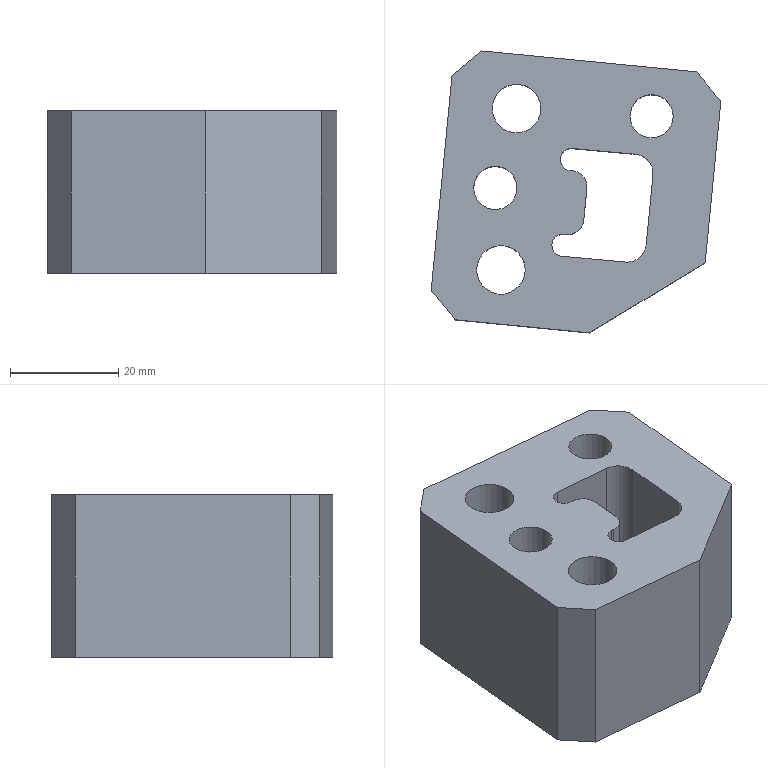Part | NX | features solid 2 | 1 solid | 30 faces | box 53.632 x 52.182 x 30 mm | volume 51476 mm3 | plane 18 | cylinder 6 | spline 6 | commonest cylinder face diameters 8 x2 9 x2 14 x2
STEP:
#1=CARTESIAN_POINT('',(-878.77,-144.615,108.));
#2=VERTEX_POINT('',#1);
#3=CARTESIAN_POINT('',(-876.165,-147.805,108.));
#4=VERTEX_POINT('',#3);
#5=CARTESIAN_POINT('',(-879.063,-147.547,108.));
#6=DIRECTION('',(0.,0.,1.));
#7=DIRECTION('',(-0.3864,-0.9223,0.));
#8=AXIS2_PLACEMENT_3D('',#5,#6,#7);
#9=ELLIPSE('',#8,2.95,2.906);
#10=EDGE_CURVE('',#2,#4,#9,.F.);
#11=ORIENTED_EDGE('',*,*,#10,.T.);
#12=CARTESIAN_POINT('',(-876.746,-153.745,108.));
#13=VERTEX_POINT('',#12);
#14=CARTESIAN_POINT('',(-873.886,-124.528,108.));
#15=DIRECTION('',(-0.09741,-0.9952,0.));
#16=VECTOR('',#15,1000.);
#17=LINE('',#14,#16);
#18=EDGE_CURVE('',#4,#13,#17,.T.);
#19=ORIENTED_EDGE('',*,*,#18,.T.);
#20=CARTESIAN_POINT('',(-879.938,-156.418,108.));
#21=VERTEX_POINT('',#20);
#22=CARTESIAN_POINT('',(-879.645,-153.487,108.));
#23=DIRECTION('',(0.,0.,1.));
#24=DIRECTION('',(-0.3864,-0.9223,0.));
#25=AXIS2_PLACEMENT_3D('',#22,#23,#24);
#26=ELLIPSE('',#25,2.95,2.906);
#27=EDGE_CURVE('',#13,#21,#26,.F.);
#28=ORIENTED_EDGE('',*,*,#27,.T.);
#29=CARTESIAN_POINT('',(-880.419,-156.374,108.));
#30=VERTEX_POINT('',#29);
#31=CARTESIAN_POINT('',(-838.877,-160.173,108.));
#32=DIRECTION('',(-0.9958,0.09106,0.));
#33=VECTOR('',#32,1000.);
#34=LINE('',#31,#33);
#35=EDGE_CURVE('',#21,#30,#34,.T.);
#36=ORIENTED_EDGE('',*,*,#35,.T.);
#37=CARTESIAN_POINT('',(-880.826,-160.449,108.));
#38=VERTEX_POINT('',#37);
#39=CARTESIAN_POINT('',(-880.622,-158.411,108.));
#40=DIRECTION('',(0.,0.,1.));
#41=DIRECTION('',(-0.3864,-0.9223,0.));
#42=AXIS2_PLACEMENT_3D('',#39,#40,#41);
#43=ELLIPSE('',#42,2.05,2.02);
#44=EDGE_CURVE('',#38,#30,#43,.F.);
#45=ORIENTED_EDGE('',*,*,#44,.F.);
#46=CARTESIAN_POINT('',(-869.041,-161.526,108.));
#47=VERTEX_POINT('',#46);
#48=CARTESIAN_POINT('',(-839.25,-164.25,108.));
#49=DIRECTION('',(-0.9958,0.09106,0.));
#50=VECTOR('',#49,1000.);
#51=LINE('',#48,#50);
#52=EDGE_CURVE('',#47,#38,#51,.T.);
#53=ORIENTED_EDGE('',*,*,#52,.F.);
#54=CARTESIAN_POINT('',(-865.2,-158.31,108.));
#55=VERTEX_POINT('',#54);
#56=CARTESIAN_POINT('',(-868.688,-157.998,108.));
#57=DIRECTION('',(0.,0.,1.));
#58=DIRECTION('',(-0.3864,-0.9223,0.));
#59=AXIS2_PLACEMENT_3D('',#56,#57,#58);
#60=ELLIPSE('',#59,3.55,3.497);
#61=EDGE_CURVE('',#55,#47,#60,.F.);
#62=ORIENTED_EDGE('',*,*,#61,.F.);
#63=CARTESIAN_POINT('',(-863.937,-145.412,108.));
#64=VERTEX_POINT('',#63);
#65=CARTESIAN_POINT('',(-862.007,-125.691,108.));
#66=DIRECTION('',(-0.09741,-0.9952,0.));
#67=VECTOR('',#66,1000.);
#68=LINE('',#65,#67);
#69=EDGE_CURVE('',#64,#55,#68,.T.);
#70=ORIENTED_EDGE('',*,*,#69,.F.);
#71=CARTESIAN_POINT('',(-867.073,-141.573,108.));
#72=VERTEX_POINT('',#71);
#73=CARTESIAN_POINT('',(-867.426,-145.101,108.));
#74=DIRECTION('',(0.,0.,1.));
#75=DIRECTION('',(-0.3864,-0.9223,0.));
#76=AXIS2_PLACEMENT_3D('',#73,#74,#75);
#77=ELLIPSE('',#76,3.55,3.497);
#78=EDGE_CURVE('',#72,#64,#77,.F.);
#79=ORIENTED_EDGE('',*,*,#78,.F.);
#80=CARTESIAN_POINT('',(-878.865,-140.495,108.));
#81=VERTEX_POINT('',#80);
#82=CARTESIAN_POINT('',(-837.425,-144.284,108.));
#83=DIRECTION('',(-0.9958,0.09106,0.));
#84=VECTOR('',#83,1000.);
#85=LINE('',#82,#84);
#86=EDGE_CURVE('',#72,#81,#85,.T.);
#87=ORIENTED_EDGE('',*,*,#86,.T.);
#88=CARTESIAN_POINT('',(-879.272,-144.569,108.));
#89=VERTEX_POINT('',#88);
#90=CARTESIAN_POINT('',(-879.068,-142.532,108.));
#91=DIRECTION('',(0.,0.,1.));
#92=DIRECTION('',(-0.3864,-0.9223,0.));
#93=AXIS2_PLACEMENT_3D('',#90,#91,#92);
#94=ELLIPSE('',#93,2.05,2.02);
#95=EDGE_CURVE('',#89,#81,#94,.F.);
#96=ORIENTED_EDGE('',*,*,#95,.F.);
#97=CARTESIAN_POINT('',(-837.798,-148.361,108.));
#98=DIRECTION('',(-0.9958,0.09106,0.));
#99=VECTOR('',#98,1000.);
#100=LINE('',#97,#99);
#101=EDGE_CURVE('',#2,#89,#100,.T.);
#102=ORIENTED_EDGE('',*,*,#101,.F.);
#103=EDGE_LOOP('',(#11,#19,#28,#36,#45,#53,#62,#70,#79,#87,#96,#102));
#104=FACE_BOUND('',#103,.T.);
#105=CARTESIAN_POINT('',(-860.199,-134.54,108.));
#106=VERTEX_POINT('',#105);
#107=CARTESIAN_POINT('',(-864.199,-134.54,108.));
#108=DIRECTION('',(0.,0.,1.));
#109=DIRECTION('',(1.,0.,0.));
#110=AXIS2_PLACEMENT_3D('',#107,#108,#109);
#111=CIRCLE('',#110,4.);
#112=EDGE_CURVE('',#106,#106,#111,.T.);
#113=ORIENTED_EDGE('',*,*,#112,.T.);
#114=EDGE_LOOP('',(#113));
#115=FACE_BOUND('',#114,.T.);
#116=CARTESIAN_POINT('',(-895.677,-122.441,108.));
#117=VERTEX_POINT('',#116);
#118=CARTESIAN_POINT('',(-855.864,-126.307,108.));
#119=VERTEX_POINT('',#118);
#120=CARTESIAN_POINT('',(-905.63,-121.474,108.));
#121=DIRECTION('',(0.9953,-0.09666,0.));
#122=VECTOR('',#121,1000.);
#123=LINE('',#120,#122);
#124=EDGE_CURVE('',#117,#119,#123,.T.);
#125=ORIENTED_EDGE('',*,*,#124,.T.);
#126=CARTESIAN_POINT('',(-851.371,-131.767,108.));
#127=VERTEX_POINT('',#126);
#128=CARTESIAN_POINT('',(-855.864,-126.307,108.));
#129=DIRECTION('',(0.6354,-0.7721,0.));
#130=VECTOR('',#129,1000.);
#131=LINE('',#128,#130);
#132=EDGE_CURVE('',#119,#127,#131,.T.);
#133=ORIENTED_EDGE('',*,*,#132,.T.);
#134=CARTESIAN_POINT('',(-854.271,-161.627,108.));
#135=VERTEX_POINT('',#134);
#136=CARTESIAN_POINT('',(-850.888,-126.79,108.));
#137=DIRECTION('',(0.09666,0.9953,0.));
#138=VECTOR('',#137,1000.);
#139=LINE('',#136,#138);
#140=EDGE_CURVE('',#135,#127,#139,.T.);
#141=ORIENTED_EDGE('',*,*,#140,.F.);
#142=CARTESIAN_POINT('',(-875.627,-174.623,108.));
#143=VERTEX_POINT('',#142);
#144=CARTESIAN_POINT('',(-875.627,-174.623,108.));
#145=DIRECTION('',(0.8542,0.5199,0.));
#146=VECTOR('',#145,1000.);
#147=LINE('',#144,#146);
#148=EDGE_CURVE('',#143,#135,#147,.T.);
#149=ORIENTED_EDGE('',*,*,#148,.F.);
#150=CARTESIAN_POINT('',(-900.51,-172.207,108.));
#151=VERTEX_POINT('',#150);
#152=CARTESIAN_POINT('',(-910.463,-171.24,108.));
#153=DIRECTION('',(0.9953,-0.09666,0.));
#154=VECTOR('',#153,1000.);
#155=LINE('',#152,#154);
#156=EDGE_CURVE('',#151,#143,#155,.T.);
#157=ORIENTED_EDGE('',*,*,#156,.F.);
#158=CARTESIAN_POINT('',(-905.003,-166.747,108.));
#159=VERTEX_POINT('',#158);
#160=CARTESIAN_POINT('',(-905.003,-166.747,108.));
#161=DIRECTION('',(-0.6354,0.7721,0.));
#162=VECTOR('',#161,1000.);
#163=LINE('',#160,#162);
#164=EDGE_CURVE('',#151,#159,#163,.T.);
#165=ORIENTED_EDGE('',*,*,#164,.T.);
#166=CARTESIAN_POINT('',(-901.137,-126.934,108.));
#167=VERTEX_POINT('',#166);
#168=CARTESIAN_POINT('',(-900.653,-121.957,108.));
#169=DIRECTION('',(0.09666,0.9953,0.));
#170=VECTOR('',#169,1000.);
#171=LINE('',#168,#170);
#172=EDGE_CURVE('',#159,#167,#171,.T.);
#173=ORIENTED_EDGE('',*,*,#172,.T.);
#174=CARTESIAN_POINT('',(-895.677,-122.441,108.));
#175=DIRECTION('',(-0.7721,-0.6354,0.));
#176=VECTOR('',#175,1000.);
#177=LINE('',#174,#176);
#178=EDGE_CURVE('',#167,#117,#177,.F.);
#179=ORIENTED_EDGE('',*,*,#178,.T.);
#180=EDGE_LOOP('',(#125,#133,#141,#149,#157,#165,#173,#179));
#181=FACE_BOUND('',#180,.T.);
#182=CARTESIAN_POINT('',(-899.078,-162.978,108.));
#183=VERTEX_POINT('',#182);
#184=CARTESIAN_POINT('',(-892.078,-162.978,108.));
#185=DIRECTION('',(0.,0.,1.));
#186=DIRECTION('',(-1.,0.,0.));
#187=AXIS2_PLACEMENT_3D('',#184,#185,#186);
#188=CIRCLE('',#187,7.);
#189=EDGE_CURVE('',#183,#183,#188,.T.);
#190=ORIENTED_EDGE('',*,*,#189,.T.);
#191=EDGE_LOOP('',(#190));
#192=FACE_BOUND('',#191,.T.);
#193=CARTESIAN_POINT('',(-896.179,-133.119,108.));
#194=VERTEX_POINT('',#193);
#195=CARTESIAN_POINT('',(-889.179,-133.119,108.));
#196=DIRECTION('',(0.,0.,1.));
#197=DIRECTION('',(-1.,0.,0.));
#198=AXIS2_PLACEMENT_3D('',#195,#196,#197);
#199=CIRCLE('',#198,7.);
#200=EDGE_CURVE('',#194,#194,#199,.T.);
#201=ORIENTED_EDGE('',*,*,#200,.T.);
#202=EDGE_LOOP('',(#201));
#203=FACE_BOUND('',#202,.T.);
#204=CARTESIAN_POINT('',(-897.117,-147.807,108.));
#205=VERTEX_POINT('',#204);
#206=CARTESIAN_POINT('',(-893.117,-147.807,108.));
#207=DIRECTION('',(0.,0.,1.));
#208=DIRECTION('',(-1.,0.,0.));
#209=AXIS2_PLACEMENT_3D('',#206,#207,#208);
#210=CIRCLE('',#209,4.);
#211=EDGE_CURVE('',#205,#205,#210,.T.);
#212=ORIENTED_EDGE('',*,*,#211,.T.);
#213=EDGE_LOOP('',(#212));
#214=FACE_BOUND('',#213,.T.);
#215=CARTESIAN_POINT('',(-835.958,-128.24,108.));
#216=DIRECTION('',(0.,0.,1.));
#217=DIRECTION('',(-1.,0.,0.));
#218=AXIS2_PLACEMENT_3D('',#215,#216,#217);
#219=PLANE('',#218);
#220=ADVANCED_FACE('',(#104,#115,#181,#192,#203,#214),#219,.F.);
#221=CARTESIAN_POINT('',(-876.746,-153.745,138.));
#222=VERTEX_POINT('',#221);
#223=CARTESIAN_POINT('',(-876.165,-147.805,138.));
#224=VERTEX_POINT('',#223);
#225=CARTESIAN_POINT('',(-876.746,-153.745,138.));
#226=DIRECTION('',(0.09741,0.9952,0.));
#227=VECTOR('',#226,1000.);
#228=LINE('',#225,#227);
#229=EDGE_CURVE('',#222,#224,#228,.T.);
#230=ORIENTED_EDGE('',*,*,#229,.T.);
#231=CARTESIAN_POINT('',(-878.77,-144.615,138.));
#232=VERTEX_POINT('',#231);
#233=CARTESIAN_POINT('',(-879.063,-147.547,138.));
#234=DIRECTION('',(0.,0.,1.));
#235=DIRECTION('',(-0.3864,-0.9223,0.));
#236=AXIS2_PLACEMENT_3D('',#233,#234,#235);
#237=ELLIPSE('',#236,2.95,2.906);
#238=EDGE_CURVE('',#224,#232,#237,.T.);
#239=ORIENTED_EDGE('',*,*,#238,.T.);
#240=CARTESIAN_POINT('',(-879.272,-144.569,138.));
#241=VERTEX_POINT('',#240);
#242=CARTESIAN_POINT('',(-879.272,-144.569,138.));
#243=DIRECTION('',(0.9958,-0.09106,0.));
#244=VECTOR('',#243,1000.);
#245=LINE('',#242,#244);
#246=EDGE_CURVE('',#241,#232,#245,.T.);
#247=ORIENTED_EDGE('',*,*,#246,.F.);
#248=CARTESIAN_POINT('',(-878.865,-140.495,138.));
#249=VERTEX_POINT('',#248);
#250=CARTESIAN_POINT('',(-879.068,-142.532,138.));
#251=DIRECTION('',(0.,0.,1.));
#252=DIRECTION('',(-0.3864,-0.9223,0.));
#253=AXIS2_PLACEMENT_3D('',#250,#251,#252);
#254=ELLIPSE('',#253,2.05,2.02);
#255=EDGE_CURVE('',#249,#241,#254,.T.);
#256=ORIENTED_EDGE('',*,*,#255,.F.);
#257=CARTESIAN_POINT('',(-867.073,-141.573,138.));
#258=VERTEX_POINT('',#257);
#259=CARTESIAN_POINT('',(-878.865,-140.495,138.));
#260=DIRECTION('',(0.9958,-0.09106,0.));
#261=VECTOR('',#260,1000.);
#262=LINE('',#259,#261);
#263=EDGE_CURVE('',#249,#258,#262,.T.);
#264=ORIENTED_EDGE('',*,*,#263,.T.);
#265=CARTESIAN_POINT('',(-863.937,-145.412,138.));
#266=VERTEX_POINT('',#265);
#267=CARTESIAN_POINT('',(-867.426,-145.101,138.));
#268=DIRECTION('',(0.,0.,1.));
#269=DIRECTION('',(-0.3864,-0.9223,0.));
#270=AXIS2_PLACEMENT_3D('',#267,#268,#269);
#271=ELLIPSE('',#270,3.55,3.497);
#272=EDGE_CURVE('',#266,#258,#271,.T.);
#273=ORIENTED_EDGE('',*,*,#272,.F.);
#274=CARTESIAN_POINT('',(-865.2,-158.31,138.));
#275=VERTEX_POINT('',#274);
#276=CARTESIAN_POINT('',(-865.2,-158.31,138.));
#277=DIRECTION('',(0.09741,0.9952,0.));
#278=VECTOR('',#277,1000.);
#279=LINE('',#276,#278);
#280=EDGE_CURVE('',#275,#266,#279,.T.);
#281=ORIENTED_EDGE('',*,*,#280,.F.);
#282=CARTESIAN_POINT('',(-869.041,-161.526,138.));
#283=VERTEX_POINT('',#282);
#284=CARTESIAN_POINT('',(-868.688,-157.998,138.));
#285=DIRECTION('',(0.,0.,1.));
#286=DIRECTION('',(-0.3864,-0.9223,0.));
#287=AXIS2_PLACEMENT_3D('',#284,#285,#286);
#288=ELLIPSE('',#287,3.55,3.497);
#289=EDGE_CURVE('',#283,#275,#288,.T.);
#290=ORIENTED_EDGE('',*,*,#289,.F.);
#291=CARTESIAN_POINT('',(-880.826,-160.449,138.));
#292=VERTEX_POINT('',#291);
#293=CARTESIAN_POINT('',(-880.826,-160.449,138.));
#294=DIRECTION('',(0.9958,-0.09106,0.));
#295=VECTOR('',#294,1000.);
#296=LINE('',#293,#295);
#297=EDGE_CURVE('',#292,#283,#296,.T.);
#298=ORIENTED_EDGE('',*,*,#297,.F.);
#299=CARTESIAN_POINT('',(-880.419,-156.374,138.));
#300=VERTEX_POINT('',#299);
#301=CARTESIAN_POINT('',(-880.622,-158.411,138.));
#302=DIRECTION('',(0.,0.,1.));
#303=DIRECTION('',(-0.3864,-0.9223,0.));
#304=AXIS2_PLACEMENT_3D('',#301,#302,#303);
#305=ELLIPSE('',#304,2.05,2.02);
#306=EDGE_CURVE('',#300,#292,#305,.T.);
#307=ORIENTED_EDGE('',*,*,#306,.F.);
#308=CARTESIAN_POINT('',(-879.938,-156.418,138.));
#309=VERTEX_POINT('',#308);
#310=CARTESIAN_POINT('',(-880.419,-156.374,138.));
#311=DIRECTION('',(0.9958,-0.09106,0.));
#312=VECTOR('',#311,1000.);
#313=LINE('',#310,#312);
#314=EDGE_CURVE('',#300,#309,#313,.T.);
#315=ORIENTED_EDGE('',*,*,#314,.T.);
#316=CARTESIAN_POINT('',(-879.645,-153.487,138.));
#317=DIRECTION('',(0.,0.,1.));
#318=DIRECTION('',(-0.3864,-0.9223,0.));
#319=AXIS2_PLACEMENT_3D('',#316,#317,#318);
#320=ELLIPSE('',#319,2.95,2.906);
#321=EDGE_CURVE('',#309,#222,#320,.T.);
#322=ORIENTED_EDGE('',*,*,#321,.T.);
#323=EDGE_LOOP('',(#230,#239,#247,#256,#264,#273,#281,#290,#298,#307,#315,#322));
#324=FACE_BOUND('',#323,.T.);
#325=CARTESIAN_POINT('',(-854.271,-161.627,138.));
#326=VERTEX_POINT('',#325);
#327=CARTESIAN_POINT('',(-851.371,-131.767,138.));
#328=VERTEX_POINT('',#327);
#329=CARTESIAN_POINT('',(-850.888,-126.79,138.));
#330=DIRECTION('',(0.09666,0.9953,0.));
#331=VECTOR('',#330,1000.);
#332=LINE('',#329,#331);
#333=EDGE_CURVE('',#326,#328,#332,.T.);
#334=ORIENTED_EDGE('',*,*,#333,.T.);
#335=CARTESIAN_POINT('',(-855.864,-126.307,138.));
#336=VERTEX_POINT('',#335);
#337=CARTESIAN_POINT('',(-846.878,-137.227,138.));
#338=DIRECTION('',(-0.6354,0.7721,0.));
#339=VECTOR('',#338,1000.);
#340=LINE('',#337,#339);
#341=EDGE_CURVE('',#328,#336,#340,.T.);
#342=ORIENTED_EDGE('',*,*,#341,.T.);
#343=CARTESIAN_POINT('',(-895.677,-122.441,138.));
#344=VERTEX_POINT('',#343);
#345=CARTESIAN_POINT('',(-905.63,-121.474,138.));
#346=DIRECTION('',(0.9953,-0.09666,0.));
#347=VECTOR('',#346,1000.);
#348=LINE('',#345,#347);
#349=EDGE_CURVE('',#344,#336,#348,.T.);
#350=ORIENTED_EDGE('',*,*,#349,.F.);
#351=CARTESIAN_POINT('',(-901.137,-126.934,138.));
#352=VERTEX_POINT('',#351);
#353=CARTESIAN_POINT('',(-862.917,-95.481,138.));
#354=DIRECTION('',(0.7721,0.6354,0.));
#355=VECTOR('',#354,1000.);
#356=LINE('',#353,#355);
#357=EDGE_CURVE('',#344,#352,#356,.F.);
#358=ORIENTED_EDGE('',*,*,#357,.T.);
#359=CARTESIAN_POINT('',(-905.003,-166.747,138.));
#360=VERTEX_POINT('',#359);
#361=CARTESIAN_POINT('',(-900.653,-121.957,138.));
#362=DIRECTION('',(0.09666,0.9953,0.));
#363=VECTOR('',#362,1000.);
#364=LINE('',#361,#363);
#365=EDGE_CURVE('',#360,#352,#364,.T.);
#366=ORIENTED_EDGE('',*,*,#365,.F.);
#367=CARTESIAN_POINT('',(-900.51,-172.207,138.));
#368=VERTEX_POINT('',#367);
#369=CARTESIAN_POINT('',(-896.016,-177.667,138.));
#370=DIRECTION('',(0.6354,-0.7721,0.));
#371=VECTOR('',#370,1000.);
#372=LINE('',#369,#371);
#373=EDGE_CURVE('',#360,#368,#372,.T.);
#374=ORIENTED_EDGE('',*,*,#373,.T.);
#375=CARTESIAN_POINT('',(-875.627,-174.623,138.));
#376=VERTEX_POINT('',#375);
#377=CARTESIAN_POINT('',(-910.463,-171.24,138.));
#378=DIRECTION('',(0.9953,-0.09666,0.));
#379=VECTOR('',#378,1000.);
#380=LINE('',#377,#379);
#381=EDGE_CURVE('',#368,#376,#380,.T.);
#382=ORIENTED_EDGE('',*,*,#381,.T.);
#383=CARTESIAN_POINT('',(-826.08,-144.471,138.));
#384=DIRECTION('',(-0.8542,-0.5199,0.));
#385=VECTOR('',#384,1000.);
#386=LINE('',#383,#385);
#387=EDGE_CURVE('',#326,#376,#386,.T.);
#388=ORIENTED_EDGE('',*,*,#387,.F.);
#389=EDGE_LOOP('',(#334,#342,#350,#358,#366,#374,#382,#388));
#390=FACE_BOUND('',#389,.T.);
#391=CARTESIAN_POINT('',(-860.199,-134.54,138.));
#392=VERTEX_POINT('',#391);
#393=CARTESIAN_POINT('',(-864.199,-134.54,138.));
#394=DIRECTION('',(0.,0.,1.));
#395=DIRECTION('',(1.,0.,0.));
#396=AXIS2_PLACEMENT_3D('',#393,#394,#395);
#397=CIRCLE('',#396,4.);
#398=EDGE_CURVE('',#392,#392,#397,.F.);
#399=ORIENTED_EDGE('',*,*,#398,.T.);
#400=EDGE_LOOP('',(#399));
#401=FACE_BOUND('',#400,.T.);
#402=CARTESIAN_POINT('',(-896.578,-162.978,138.));
#403=VERTEX_POINT('',#402);
#404=CARTESIAN_POINT('',(-892.078,-162.978,138.));
#405=DIRECTION('',(0.,0.,1.));
#406=DIRECTION('',(-1.,0.,0.));
#407=AXIS2_PLACEMENT_3D('',#404,#405,#406);
#408=CIRCLE('',#407,4.5);
#409=EDGE_CURVE('',#403,#403,#408,.T.);
#410=ORIENTED_EDGE('',*,*,#409,.F.);
#411=EDGE_LOOP('',(#410));
#412=FACE_BOUND('',#411,.T.);
#413=CARTESIAN_POINT('',(-893.679,-133.119,138.));
#414=VERTEX_POINT('',#413);
#415=CARTESIAN_POINT('',(-889.179,-133.119,138.));
#416=DIRECTION('',(0.,0.,1.));
#417=DIRECTION('',(-1.,0.,0.));
#418=AXIS2_PLACEMENT_3D('',#415,#416,#417);
#419=CIRCLE('',#418,4.5);
#420=EDGE_CURVE('',#414,#414,#419,.T.);
#421=ORIENTED_EDGE('',*,*,#420,.F.);
#422=EDGE_LOOP('',(#421));
#423=FACE_BOUND('',#422,.T.);
#424=CARTESIAN_POINT('',(-897.117,-147.807,138.));
#425=VERTEX_POINT('',#424);
#426=CARTESIAN_POINT('',(-893.117,-147.807,138.));
#427=DIRECTION('',(0.,0.,1.));
#428=DIRECTION('',(-1.,0.,0.));
#429=AXIS2_PLACEMENT_3D('',#426,#427,#428);
#430=CIRCLE('',#429,4.);
#431=EDGE_CURVE('',#425,#425,#430,.T.);
#432=ORIENTED_EDGE('',*,*,#431,.F.);
#433=EDGE_LOOP('',(#432));
#434=FACE_BOUND('',#433,.T.);
#435=CARTESIAN_POINT('',(-835.958,-128.24,138.));
#436=DIRECTION('',(0.,0.,1.));
#437=DIRECTION('',(-1.,0.,0.));
#438=AXIS2_PLACEMENT_3D('',#435,#436,#437);
#439=PLANE('',#438);
#440=ADVANCED_FACE('',(#324,#390,#401,#412,#423,#434),#439,.T.);
#441=ORIENTED_EDGE('',*,*,#349,.T.);
#442=CARTESIAN_POINT('',(-855.864,-126.307,108.));
#443=DIRECTION('',(0.,0.,-1.));
#444=VECTOR('',#443,1000.);
#445=LINE('',#442,#444);
#446=EDGE_CURVE('',#336,#119,#445,.T.);
#447=ORIENTED_EDGE('',*,*,#446,.T.);
#448=ORIENTED_EDGE('',*,*,#124,.F.);
#449=CARTESIAN_POINT('',(-895.677,-122.441,108.));
#450=DIRECTION('',(0.,0.,1.));
#451=VECTOR('',#450,1000.);
#452=LINE('',#449,#451);
#453=EDGE_CURVE('',#117,#344,#452,.T.);
#454=ORIENTED_EDGE('',*,*,#453,.T.);
#455=EDGE_LOOP('',(#441,#447,#448,#454));
#456=FACE_BOUND('',#455,.T.);
#457=CARTESIAN_POINT('',(-900.653,-121.957,108.));
#458=DIRECTION('',(-0.09666,-0.9953,0.));
#459=DIRECTION('',(0.9953,-0.09666,0.));
#460=AXIS2_PLACEMENT_3D('',#457,#458,#459);
#461=PLANE('',#460);
#462=ADVANCED_FACE('',(#456),#461,.F.);
#463=ORIENTED_EDGE('',*,*,#140,.T.);
#464=CARTESIAN_POINT('',(-851.371,-131.767,138.));
#465=DIRECTION('',(0.,0.,1.));
#466=VECTOR('',#465,1000.);
#467=LINE('',#464,#466);
#468=EDGE_CURVE('',#127,#328,#467,.T.);
#469=ORIENTED_EDGE('',*,*,#468,.T.);
#470=ORIENTED_EDGE('',*,*,#333,.F.);
#471=CARTESIAN_POINT('',(-854.271,-161.627,308.));
#472=DIRECTION('',(0.,0.,-1.));
#473=VECTOR('',#472,1000.);
#474=LINE('',#471,#473);
#475=EDGE_CURVE('',#326,#135,#474,.T.);
#476=ORIENTED_EDGE('',*,*,#475,.T.);
#477=EDGE_LOOP('',(#463,#469,#470,#476));
#478=FACE_BOUND('',#477,.T.);
#479=CARTESIAN_POINT('',(-855.72,-176.556,108.));
#480=DIRECTION('',(0.9953,-0.09666,0.));
#481=DIRECTION('',(0.09666,0.9953,0.));
#482=AXIS2_PLACEMENT_3D('',#479,#480,#481);
#483=PLANE('',#482);
#484=ADVANCED_FACE('',(#478),#483,.T.);
#485=CARTESIAN_POINT('',(-875.627,-174.623,308.));
#486=DIRECTION('',(0.,0.,-1.));
#487=VECTOR('',#486,1000.);
#488=LINE('',#485,#487);
#489=EDGE_CURVE('',#376,#143,#488,.T.);
#490=ORIENTED_EDGE('',*,*,#489,.F.);
#491=ORIENTED_EDGE('',*,*,#381,.F.);
#492=CARTESIAN_POINT('',(-900.51,-172.207,108.));
#493=DIRECTION('',(0.,0.,-1.));
#494=VECTOR('',#493,1000.);
#495=LINE('',#492,#494);
#496=EDGE_CURVE('',#368,#151,#495,.T.);
#497=ORIENTED_EDGE('',*,*,#496,.T.);
#498=ORIENTED_EDGE('',*,*,#156,.T.);
#499=EDGE_LOOP('',(#490,#491,#497,#498));
#500=FACE_BOUND('',#499,.T.);
#501=CARTESIAN_POINT('',(-905.486,-171.723,108.));
#502=DIRECTION('',(-0.09666,-0.9953,0.));
#503=DIRECTION('',(0.9953,-0.09666,0.));
#504=AXIS2_PLACEMENT_3D('',#501,#502,#503);
#505=PLANE('',#504);
#506=ADVANCED_FACE('',(#500),#505,.T.);
#507=ORIENTED_EDGE('',*,*,#172,.F.);
#508=CARTESIAN_POINT('',(-905.003,-166.747,138.));
#509=DIRECTION('',(0.,0.,1.));
#510=VECTOR('',#509,1000.);
#511=LINE('',#508,#510);
#512=EDGE_CURVE('',#159,#360,#511,.T.);
#513=ORIENTED_EDGE('',*,*,#512,.T.);
#514=ORIENTED_EDGE('',*,*,#365,.T.);
#515=CARTESIAN_POINT('',(-901.137,-126.934,108.));
#516=DIRECTION('',(0.,0.,-1.));
#517=VECTOR('',#516,1000.);
#518=LINE('',#515,#517);
#519=EDGE_CURVE('',#352,#167,#518,.T.);
#520=ORIENTED_EDGE('',*,*,#519,.T.);
#521=EDGE_LOOP('',(#507,#513,#514,#520));
#522=FACE_BOUND('',#521,.T.);
#523=CARTESIAN_POINT('',(-905.486,-171.723,108.));
#524=DIRECTION('',(0.9953,-0.09666,0.));
#525=DIRECTION('',(0.09666,0.9953,0.));
#526=AXIS2_PLACEMENT_3D('',#523,#524,#525);
#527=PLANE('',#526);
#528=ADVANCED_FACE('',(#522),#527,.F.);
#529=CARTESIAN_POINT('',(-885.209,-164.325,123.));
#530=VERTEX_POINT('',#529);
#531=CARTESIAN_POINT('',(-892.078,-162.978,123.));
#532=DIRECTION('',(0.,0.,-1.));
#533=DIRECTION('',(0.9813,-0.1924,0.));
#534=AXIS2_PLACEMENT_3D('',#531,#532,#533);
#535=CIRCLE('',#534,7.);
#536=EDGE_CURVE('',#530,#530,#535,.T.);
#537=ORIENTED_EDGE('',*,*,#536,.F.);
#538=EDGE_LOOP('',(#537));
#539=FACE_BOUND('',#538,.T.);
#540=ORIENTED_EDGE('',*,*,#189,.F.);
#541=EDGE_LOOP('',(#540));
#542=FACE_BOUND('',#541,.T.);
#543=CARTESIAN_POINT('',(-892.078,-162.978,123.));
#544=DIRECTION('',(0.,0.,-1.));
#545=DIRECTION('',(0.9813,-0.1924,0.));
#546=AXIS2_PLACEMENT_3D('',#543,#544,#545);
#547=CYLINDRICAL_SURFACE('',#546,7.);
#548=ADVANCED_FACE('',(#539,#542),#547,.F.);
#549=CARTESIAN_POINT('',(-896.578,-162.978,123.));
#550=VERTEX_POINT('',#549);
#551=CARTESIAN_POINT('',(-892.078,-162.978,123.));
#552=DIRECTION('',(0.,0.,1.));
#553=DIRECTION('',(-1.,0.,0.));
#554=AXIS2_PLACEMENT_3D('',#551,#552,#553);
#555=CIRCLE('',#554,4.5);
#556=EDGE_CURVE('',#550,#550,#555,.T.);
#557=ORIENTED_EDGE('',*,*,#556,.T.);
#558=EDGE_LOOP('',(#557));
#559=FACE_BOUND('',#558,.T.);
#560=ORIENTED_EDGE('',*,*,#536,.T.);
#561=EDGE_LOOP('',(#560));
#562=FACE_BOUND('',#561,.T.);
#563=CARTESIAN_POINT('',(-892.078,-162.978,123.));
#564=DIRECTION('',(0.,0.,1.));
#565=DIRECTION('',(-0.9813,0.1924,0.));
#566=AXIS2_PLACEMENT_3D('',#563,#564,#565);
#567=PLANE('',#566);
#568=ADVANCED_FACE('',(#559,#562),#567,.F.);
#569=ORIENTED_EDGE('',*,*,#409,.T.);
#570=EDGE_LOOP('',(#569));
#571=FACE_BOUND('',#570,.T.);
#572=ORIENTED_EDGE('',*,*,#556,.F.);
#573=EDGE_LOOP('',(#572));
#574=FACE_BOUND('',#573,.T.);
#575=CARTESIAN_POINT('',(-892.078,-162.978,123.));
#576=DIRECTION('',(0.,0.,1.));
#577=DIRECTION('',(-0.9813,0.1924,0.));
#578=AXIS2_PLACEMENT_3D('',#575,#576,#577);
#579=CYLINDRICAL_SURFACE('',#578,4.5);
#580=ADVANCED_FACE('',(#571,#574),#579,.F.);
#581=CARTESIAN_POINT('',(-882.309,-134.466,123.));
#582=VERTEX_POINT('',#581);
#583=CARTESIAN_POINT('',(-889.179,-133.119,123.));
#584=DIRECTION('',(0.,0.,-1.));
#585=DIRECTION('',(0.9813,-0.1924,0.));
#586=AXIS2_PLACEMENT_3D('',#583,#584,#585);
#587=CIRCLE('',#586,7.);
#588=EDGE_CURVE('',#582,#582,#587,.T.);
#589=ORIENTED_EDGE('',*,*,#588,.F.);
#590=EDGE_LOOP('',(#589));
#591=FACE_BOUND('',#590,.T.);
#592=ORIENTED_EDGE('',*,*,#200,.F.);
#593=EDGE_LOOP('',(#592));
#594=FACE_BOUND('',#593,.T.);
#595=CARTESIAN_POINT('',(-889.179,-133.119,123.));
#596=DIRECTION('',(0.,0.,-1.));
#597=DIRECTION('',(0.9813,-0.1924,0.));
#598=AXIS2_PLACEMENT_3D('',#595,#596,#597);
#599=CYLINDRICAL_SURFACE('',#598,7.);
#600=ADVANCED_FACE('',(#591,#594),#599,.F.);
#601=CARTESIAN_POINT('',(-893.679,-133.119,123.));
#602=VERTEX_POINT('',#601);
#603=CARTESIAN_POINT('',(-889.179,-133.119,123.));
#604=DIRECTION('',(0.,0.,1.));
#605=DIRECTION('',(-1.,0.,0.));
#606=AXIS2_PLACEMENT_3D('',#603,#604,#605);
#607=CIRCLE('',#606,4.5);
#608=EDGE_CURVE('',#602,#602,#607,.T.);
#609=ORIENTED_EDGE('',*,*,#608,.T.);
#610=EDGE_LOOP('',(#609));
#611=FACE_BOUND('',#610,.T.);
#612=ORIENTED_EDGE('',*,*,#588,.T.);
#613=EDGE_LOOP('',(#612));
#614=FACE_BOUND('',#613,.T.);
#615=CARTESIAN_POINT('',(-889.179,-133.119,123.));
#616=DIRECTION('',(0.,0.,1.));
#617=DIRECTION('',(-0.9813,0.1924,0.));
#618=AXIS2_PLACEMENT_3D('',#615,#616,#617);
#619=PLANE('',#618);
#620=ADVANCED_FACE('',(#611,#614),#619,.F.);
#621=ORIENTED_EDGE('',*,*,#420,.T.);
#622=EDGE_LOOP('',(#621));
#623=FACE_BOUND('',#622,.T.);
#624=ORIENTED_EDGE('',*,*,#608,.F.);
#625=EDGE_LOOP('',(#624));
#626=FACE_BOUND('',#625,.T.);
#627=CARTESIAN_POINT('',(-889.179,-133.119,123.));
#628=DIRECTION('',(0.,0.,1.));
#629=DIRECTION('',(-0.9813,0.1924,0.));
#630=AXIS2_PLACEMENT_3D('',#627,#628,#629);
#631=CYLINDRICAL_SURFACE('',#630,4.5);
#632=ADVANCED_FACE('',(#623,#626),#631,.F.);
#633=ORIENTED_EDGE('',*,*,#431,.T.);
#634=EDGE_LOOP('',(#633));
#635=FACE_BOUND('',#634,.T.);
#636=ORIENTED_EDGE('',*,*,#211,.F.);
#637=EDGE_LOOP('',(#636));
#638=FACE_BOUND('',#637,.T.);
#639=CARTESIAN_POINT('',(-893.117,-147.807,148.));
#640=DIRECTION('',(0.,0.,-1.));
#641=DIRECTION('',(1.,0.,0.));
#642=AXIS2_PLACEMENT_3D('',#639,#640,#641);
#643=CYLINDRICAL_SURFACE('',#642,4.);
#644=ADVANCED_FACE('',(#635,#638),#643,.F.);
#645=ORIENTED_EDGE('',*,*,#164,.F.);
#646=ORIENTED_EDGE('',*,*,#496,.F.);
#647=ORIENTED_EDGE('',*,*,#373,.F.);
#648=ORIENTED_EDGE('',*,*,#512,.F.);
#649=EDGE_LOOP('',(#645,#646,#647,#648));
#650=FACE_BOUND('',#649,.T.);
#651=CARTESIAN_POINT('',(-905.003,-166.747,108.));
#652=DIRECTION('',(-0.7721,-0.6354,0.));
#653=DIRECTION('',(0.6354,-0.7721,0.));
#654=AXIS2_PLACEMENT_3D('',#651,#652,#653);
#655=PLANE('',#654);
#656=ADVANCED_FACE('',(#650),#655,.T.);
#657=ORIENTED_EDGE('',*,*,#178,.F.);
#658=ORIENTED_EDGE('',*,*,#519,.F.);
#659=ORIENTED_EDGE('',*,*,#357,.F.);
#660=ORIENTED_EDGE('',*,*,#453,.F.);
#661=EDGE_LOOP('',(#657,#658,#659,#660));
#662=FACE_BOUND('',#661,.T.);
#663=CARTESIAN_POINT('',(-895.677,-122.441,108.));
#664=DIRECTION('',(0.6354,-0.7721,0.));
#665=DIRECTION('',(0.7721,0.6354,0.));
#666=AXIS2_PLACEMENT_3D('',#663,#664,#665);
#667=PLANE('',#666);
#668=ADVANCED_FACE('',(#662),#667,.F.);
#669=ORIENTED_EDGE('',*,*,#398,.F.);
#670=EDGE_LOOP('',(#669));
#671=FACE_BOUND('',#670,.T.);
#672=ORIENTED_EDGE('',*,*,#112,.F.);
#673=EDGE_LOOP('',(#672));
#674=FACE_BOUND('',#673,.T.);
#675=CARTESIAN_POINT('',(-864.199,-134.54,188.));
#676=DIRECTION('',(0.,0.,-1.));
#677=DIRECTION('',(1.,0.,0.));
#678=AXIS2_PLACEMENT_3D('',#675,#676,#677);
#679=CYLINDRICAL_SURFACE('',#678,4.);
#680=ADVANCED_FACE('',(#671,#674),#679,.F.);
#681=ORIENTED_EDGE('',*,*,#387,.T.);
#682=ORIENTED_EDGE('',*,*,#489,.T.);
#683=ORIENTED_EDGE('',*,*,#148,.T.);
#684=ORIENTED_EDGE('',*,*,#475,.F.);
#685=EDGE_LOOP('',(#681,#682,#683,#684));
#686=FACE_BOUND('',#685,.T.);
#687=CARTESIAN_POINT('',(-875.627,-174.623,308.));
#688=DIRECTION('',(-0.5199,0.8542,0.));
#689=DIRECTION('',(-0.8542,-0.5199,0.));
#690=AXIS2_PLACEMENT_3D('',#687,#688,#689);
#691=PLANE('',#690);
#692=ADVANCED_FACE('',(#686),#691,.F.);
#693=ORIENTED_EDGE('',*,*,#341,.F.);
#694=ORIENTED_EDGE('',*,*,#468,.F.);
#695=ORIENTED_EDGE('',*,*,#132,.F.);
#696=ORIENTED_EDGE('',*,*,#446,.F.);
#697=EDGE_LOOP('',(#693,#694,#695,#696));
#698=FACE_BOUND('',#697,.T.);
#699=CARTESIAN_POINT('',(-855.864,-126.307,108.));
#700=DIRECTION('',(0.7721,0.6354,0.));
#701=DIRECTION('',(-0.6354,0.7721,0.));
#702=AXIS2_PLACEMENT_3D('',#699,#700,#701);
#703=PLANE('',#702);
#704=ADVANCED_FACE('',(#698),#703,.T.);
#705=CARTESIAN_POINT('',(-876.165,-147.805,211.));
#706=DIRECTION('',(0.,0.,-1.));
#707=VECTOR('',#706,1000.);
#708=LINE('',#705,#707);
#709=EDGE_CURVE('',#224,#4,#708,.T.);
#710=ORIENTED_EDGE('',*,*,#709,.F.);
#711=ORIENTED_EDGE('',*,*,#229,.F.);
#712=CARTESIAN_POINT('',(-876.746,-153.745,211.));
#713=DIRECTION('',(0.,0.,-1.));
#714=VECTOR('',#713,1000.);
#715=LINE('',#712,#714);
#716=EDGE_CURVE('',#222,#13,#715,.T.);
#717=ORIENTED_EDGE('',*,*,#716,.T.);
#718=ORIENTED_EDGE('',*,*,#18,.F.);
#719=EDGE_LOOP('',(#710,#711,#717,#718));
#720=FACE_BOUND('',#719,.T.);
#721=CARTESIAN_POINT('',(-876.746,-153.745,211.));
#722=DIRECTION('',(-0.9952,0.09741,0.));
#723=DIRECTION('',(-0.09741,-0.9952,0.));
#724=AXIS2_PLACEMENT_3D('',#721,#722,#723);
#725=PLANE('',#724);
#726=ADVANCED_FACE('',(#720),#725,.F.);
#727=ORIENTED_EDGE('',*,*,#716,.F.);
#728=ORIENTED_EDGE('',*,*,#321,.F.);
#729=CARTESIAN_POINT('',(-879.938,-156.418,211.));
#730=DIRECTION('',(0.,0.,-1.));
#731=VECTOR('',#730,1000.);
#732=LINE('',#729,#731);
#733=EDGE_CURVE('',#309,#21,#732,.T.);
#734=ORIENTED_EDGE('',*,*,#733,.T.);
#735=ORIENTED_EDGE('',*,*,#27,.F.);
#736=EDGE_LOOP('',(#727,#728,#734,#735));
#737=FACE_BOUND('',#736,.T.);
#738=CARTESIAN_POINT('',(-879.938,-156.418,138.));
#739=CARTESIAN_POINT('',(-879.938,-156.418,108.));
#740=CARTESIAN_POINT('',(-879.174,-156.488,138.));
#741=CARTESIAN_POINT('',(-879.174,-156.488,108.));
#742=CARTESIAN_POINT('',(-877.587,-155.982,138.));
#743=CARTESIAN_POINT('',(-877.587,-155.982,108.));
#744=CARTESIAN_POINT('',(-876.812,-154.492,138.));
#745=CARTESIAN_POINT('',(-876.812,-154.492,108.));
#746=CARTESIAN_POINT('',(-876.744,-153.718,138.));
#747=CARTESIAN_POINT('',(-876.744,-153.718,108.));
#748=B_SPLINE_SURFACE_WITH_KNOTS('',3,1,((#738,#739),(#740,#741),(#742,#743),(#744,#745),(#746,#747)),.SURF_OF_LINEAR_EXTRUSION.,.F.,.F.,.F.,(4,1,4),(2,2),(0.3012,1.092,1.884),(0.,1.),.UNSPECIFIED.);
#749=ADVANCED_FACE('',(#737),#748,.F.);
#750=ORIENTED_EDGE('',*,*,#733,.F.);
#751=ORIENTED_EDGE('',*,*,#314,.F.);
#752=CARTESIAN_POINT('',(-880.419,-156.374,211.));
#753=DIRECTION('',(0.,0.,-1.));
#754=VECTOR('',#753,1000.);
#755=LINE('',#752,#754);
#756=EDGE_CURVE('',#300,#30,#755,.T.);
#757=ORIENTED_EDGE('',*,*,#756,.T.);
#758=ORIENTED_EDGE('',*,*,#35,.F.);
#759=EDGE_LOOP('',(#750,#751,#757,#758));
#760=FACE_BOUND('',#759,.T.);
#761=CARTESIAN_POINT('',(-880.419,-156.374,211.));
#762=DIRECTION('',(0.09106,0.9958,0.));
#763=DIRECTION('',(-0.9958,0.09106,0.));
#764=AXIS2_PLACEMENT_3D('',#761,#762,#763);
#765=PLANE('',#764);
#766=ADVANCED_FACE('',(#760),#765,.F.);
#767=ORIENTED_EDGE('',*,*,#44,.T.);
#768=ORIENTED_EDGE('',*,*,#756,.F.);
#769=ORIENTED_EDGE('',*,*,#306,.T.);
#770=CARTESIAN_POINT('',(-880.826,-160.449,211.));
#771=DIRECTION('',(0.,0.,-1.));
#772=VECTOR('',#771,1000.);
#773=LINE('',#770,#772);
#774=EDGE_CURVE('',#292,#38,#773,.T.);
#775=ORIENTED_EDGE('',*,*,#774,.T.);
#776=EDGE_LOOP('',(#767,#768,#769,#775));
#777=FACE_BOUND('',#776,.T.);
#778=CARTESIAN_POINT('',(-880.381,-156.378,138.));
#779=CARTESIAN_POINT('',(-880.381,-156.378,108.));
#780=CARTESIAN_POINT('',(-880.91,-156.319,138.));
#781=CARTESIAN_POINT('',(-880.91,-156.319,108.));
#782=CARTESIAN_POINT('',(-882.017,-156.648,138.));
#783=CARTESIAN_POINT('',(-882.017,-156.648,108.));
#784=CARTESIAN_POINT('',(-882.855,-158.186,138.));
#785=CARTESIAN_POINT('',(-882.855,-158.186,108.));
#786=CARTESIAN_POINT('',(-882.368,-159.857,138.));
#787=CARTESIAN_POINT('',(-882.368,-159.857,108.));
#788=CARTESIAN_POINT('',(-881.357,-160.4,138.));
#789=CARTESIAN_POINT('',(-881.357,-160.4,108.));
#790=CARTESIAN_POINT('',(-880.826,-160.449,138.));
#791=CARTESIAN_POINT('',(-880.826,-160.449,108.));
#792=B_SPLINE_SURFACE_WITH_KNOTS('',3,1,((#778,#779),(#780,#781),(#782,#783),(#784,#785),(#786,#787),(#788,#789),(#790,#791)),.SURF_OF_LINEAR_EXTRUSION.,.F.,.F.,.F.,(4,1,1,1,4),(2,2),(3.424,4.214,5.004,5.794,6.584),(0.,1.),.UNSPECIFIED.);
#793=ADVANCED_FACE('',(#777),#792,.T.);
#794=ORIENTED_EDGE('',*,*,#52,.T.);
#795=ORIENTED_EDGE('',*,*,#774,.F.);
#796=ORIENTED_EDGE('',*,*,#297,.T.);
#797=CARTESIAN_POINT('',(-869.041,-161.526,211.));
#798=DIRECTION('',(0.,0.,-1.));
#799=VECTOR('',#798,1000.);
#800=LINE('',#797,#799);
#801=EDGE_CURVE('',#283,#47,#800,.T.);
#802=ORIENTED_EDGE('',*,*,#801,.T.);
#803=EDGE_LOOP('',(#794,#795,#796,#802));
#804=FACE_BOUND('',#803,.T.);
#805=CARTESIAN_POINT('',(-880.826,-160.449,211.));
#806=DIRECTION('',(0.09106,0.9958,0.));
#807=DIRECTION('',(-0.9958,0.09106,0.));
#808=AXIS2_PLACEMENT_3D('',#805,#806,#807);
#809=PLANE('',#808);
#810=ADVANCED_FACE('',(#804),#809,.T.);
#811=ORIENTED_EDGE('',*,*,#61,.T.);
#812=ORIENTED_EDGE('',*,*,#801,.F.);
#813=ORIENTED_EDGE('',*,*,#289,.T.);
#814=CARTESIAN_POINT('',(-865.2,-158.31,211.));
#815=DIRECTION('',(0.,0.,-1.));
#816=VECTOR('',#815,1000.);
#817=LINE('',#814,#816);
#818=EDGE_CURVE('',#275,#55,#817,.T.);
#819=ORIENTED_EDGE('',*,*,#818,.T.);
#820=EDGE_LOOP('',(#811,#812,#813,#819));
#821=FACE_BOUND('',#820,.T.);
#822=CARTESIAN_POINT('',(-869.074,-161.523,138.));
#823=CARTESIAN_POINT('',(-869.074,-161.523,108.));
#824=CARTESIAN_POINT('',(-868.155,-161.616,138.));
#825=CARTESIAN_POINT('',(-868.155,-161.616,108.));
#826=CARTESIAN_POINT('',(-866.24,-161.025,138.));
#827=CARTESIAN_POINT('',(-866.24,-161.025,108.));
#828=CARTESIAN_POINT('',(-865.291,-159.24,138.));
#829=CARTESIAN_POINT('',(-865.291,-159.24,108.));
#830=CARTESIAN_POINT('',(-865.2,-158.31,138.));
#831=CARTESIAN_POINT('',(-865.2,-158.31,108.));
#832=B_SPLINE_SURFACE_WITH_KNOTS('',3,1,((#822,#823),(#824,#825),(#826,#827),(#828,#829),(#830,#831)),.SURF_OF_LINEAR_EXTRUSION.,.F.,.F.,.F.,(4,1,4),(2,2),(0.2918,1.083,1.874),(0.,1.),.UNSPECIFIED.);
#833=ADVANCED_FACE('',(#821),#832,.T.);
#834=ORIENTED_EDGE('',*,*,#69,.T.);
#835=ORIENTED_EDGE('',*,*,#818,.F.);
#836=ORIENTED_EDGE('',*,*,#280,.T.);
#837=CARTESIAN_POINT('',(-863.937,-145.412,211.));
#838=DIRECTION('',(0.,0.,-1.));
#839=VECTOR('',#838,1000.);
#840=LINE('',#837,#839);
#841=EDGE_CURVE('',#266,#64,#840,.T.);
#842=ORIENTED_EDGE('',*,*,#841,.T.);
#843=EDGE_LOOP('',(#834,#835,#836,#842));
#844=FACE_BOUND('',#843,.T.);
#845=CARTESIAN_POINT('',(-865.2,-158.31,211.));
#846=DIRECTION('',(-0.9952,0.09741,0.));
#847=DIRECTION('',(-0.09741,-0.9952,0.));
#848=AXIS2_PLACEMENT_3D('',#845,#846,#847);
#849=PLANE('',#848);
#850=ADVANCED_FACE('',(#844),#849,.T.);
#851=ORIENTED_EDGE('',*,*,#78,.T.);
#852=ORIENTED_EDGE('',*,*,#841,.F.);
#853=ORIENTED_EDGE('',*,*,#272,.T.);
#854=CARTESIAN_POINT('',(-867.073,-141.573,211.));
#855=DIRECTION('',(0.,0.,-1.));
#856=VECTOR('',#855,1000.);
#857=LINE('',#854,#856);
#858=EDGE_CURVE('',#258,#72,#857,.T.);
#859=ORIENTED_EDGE('',*,*,#858,.T.);
#860=EDGE_LOOP('',(#851,#852,#853,#859));
#861=FACE_BOUND('',#860,.T.);
#862=CARTESIAN_POINT('',(-863.941,-145.445,138.));
#863=CARTESIAN_POINT('',(-863.941,-145.445,108.));
#864=CARTESIAN_POINT('',(-863.841,-144.518,138.));
#865=CARTESIAN_POINT('',(-863.841,-144.518,108.));
#866=CARTESIAN_POINT('',(-864.406,-142.596,138.));
#867=CARTESIAN_POINT('',(-864.406,-142.596,108.));
#868=CARTESIAN_POINT('',(-866.156,-141.657,138.));
#869=CARTESIAN_POINT('',(-866.156,-141.657,108.));
#870=CARTESIAN_POINT('',(-867.073,-141.573,138.));
#871=CARTESIAN_POINT('',(-867.073,-141.573,108.));
#872=B_SPLINE_SURFACE_WITH_KNOTS('',3,1,((#862,#863),(#864,#865),(#866,#867),(#868,#869),(#870,#871)),.SURF_OF_LINEAR_EXTRUSION.,.F.,.F.,.F.,(4,1,4),(2,2),(1.865,2.654,3.443),(0.,1.),.UNSPECIFIED.);
#873=ADVANCED_FACE('',(#861),#872,.T.);
#874=ORIENTED_EDGE('',*,*,#858,.F.);
#875=ORIENTED_EDGE('',*,*,#263,.F.);
#876=CARTESIAN_POINT('',(-878.865,-140.495,211.));
#877=DIRECTION('',(0.,0.,-1.));
#878=VECTOR('',#877,1000.);
#879=LINE('',#876,#878);
#880=EDGE_CURVE('',#249,#81,#879,.T.);
#881=ORIENTED_EDGE('',*,*,#880,.T.);
#882=ORIENTED_EDGE('',*,*,#86,.F.);
#883=EDGE_LOOP('',(#874,#875,#881,#882));
#884=FACE_BOUND('',#883,.T.);
#885=CARTESIAN_POINT('',(-878.865,-140.495,211.));
#886=DIRECTION('',(0.09106,0.9958,0.));
#887=DIRECTION('',(-0.9958,0.09106,0.));
#888=AXIS2_PLACEMENT_3D('',#885,#886,#887);
#889=PLANE('',#888);
#890=ADVANCED_FACE('',(#884),#889,.F.);
#891=ORIENTED_EDGE('',*,*,#95,.T.);
#892=ORIENTED_EDGE('',*,*,#880,.F.);
#893=ORIENTED_EDGE('',*,*,#255,.T.);
#894=CARTESIAN_POINT('',(-879.272,-144.569,211.));
#895=DIRECTION('',(0.,0.,-1.));
#896=VECTOR('',#895,1000.);
#897=LINE('',#894,#896);
#898=EDGE_CURVE('',#241,#89,#897,.T.);
#899=ORIENTED_EDGE('',*,*,#898,.T.);
#900=EDGE_LOOP('',(#891,#892,#893,#899));
#901=FACE_BOUND('',#900,.T.);
#902=CARTESIAN_POINT('',(-878.827,-140.499,138.));
#903=CARTESIAN_POINT('',(-878.827,-140.499,108.));
#904=CARTESIAN_POINT('',(-879.356,-140.44,138.));
#905=CARTESIAN_POINT('',(-879.356,-140.44,108.));
#906=CARTESIAN_POINT('',(-880.463,-140.769,138.));
#907=CARTESIAN_POINT('',(-880.463,-140.769,108.));
#908=CARTESIAN_POINT('',(-881.301,-142.306,138.));
#909=CARTESIAN_POINT('',(-881.301,-142.306,108.));
#910=CARTESIAN_POINT('',(-880.814,-143.978,138.));
#911=CARTESIAN_POINT('',(-880.814,-143.978,108.));
#912=CARTESIAN_POINT('',(-879.802,-144.521,138.));
#913=CARTESIAN_POINT('',(-879.802,-144.521,108.));
#914=CARTESIAN_POINT('',(-879.272,-144.569,138.));
#915=CARTESIAN_POINT('',(-879.272,-144.569,108.));
#916=B_SPLINE_SURFACE_WITH_KNOTS('',3,1,((#902,#903),(#904,#905),(#906,#907),(#908,#909),(#910,#911),(#912,#913),(#914,#915)),.SURF_OF_LINEAR_EXTRUSION.,.F.,.F.,.F.,(4,1,1,1,4),(2,2),(3.424,4.214,5.004,5.794,6.584),(0.,1.),.UNSPECIFIED.);
#917=ADVANCED_FACE('',(#901),#916,.T.);
#918=ORIENTED_EDGE('',*,*,#101,.T.);
#919=ORIENTED_EDGE('',*,*,#898,.F.);
#920=ORIENTED_EDGE('',*,*,#246,.T.);
#921=CARTESIAN_POINT('',(-878.77,-144.615,211.));
#922=DIRECTION('',(0.,0.,-1.));
#923=VECTOR('',#922,1000.);
#924=LINE('',#921,#923);
#925=EDGE_CURVE('',#232,#2,#924,.T.);
#926=ORIENTED_EDGE('',*,*,#925,.T.);
#927=EDGE_LOOP('',(#918,#919,#920,#926));
#928=FACE_BOUND('',#927,.T.);
#929=CARTESIAN_POINT('',(-879.272,-144.569,211.));
#930=DIRECTION('',(0.09106,0.9958,0.));
#931=DIRECTION('',(-0.9958,0.09106,0.));
#932=AXIS2_PLACEMENT_3D('',#929,#930,#931);
#933=PLANE('',#932);
#934=ADVANCED_FACE('',(#928),#933,.T.);
#935=ORIENTED_EDGE('',*,*,#925,.F.);
#936=ORIENTED_EDGE('',*,*,#238,.F.);
#937=ORIENTED_EDGE('',*,*,#709,.T.);
#938=ORIENTED_EDGE('',*,*,#10,.F.);
#939=EDGE_LOOP('',(#935,#936,#937,#938));
#940=FACE_BOUND('',#939,.T.);
#941=CARTESIAN_POINT('',(-876.165,-147.805,138.));
#942=CARTESIAN_POINT('',(-876.165,-147.805,108.));
#943=CARTESIAN_POINT('',(-876.089,-147.034,138.));
#944=CARTESIAN_POINT('',(-876.089,-147.034,108.));
#945=CARTESIAN_POINT('',(-876.573,-145.441,138.));
#946=CARTESIAN_POINT('',(-876.573,-145.441,108.));
#947=CARTESIAN_POINT('',(-878.035,-144.675,138.));
#948=CARTESIAN_POINT('',(-878.035,-144.675,108.));
#949=CARTESIAN_POINT('',(-878.798,-144.613,138.));
#950=CARTESIAN_POINT('',(-878.798,-144.613,108.));
#951=B_SPLINE_SURFACE_WITH_KNOTS('',3,1,((#941,#942),(#943,#944),(#945,#946),(#947,#948),(#949,#950)),.SURF_OF_LINEAR_EXTRUSION.,.F.,.F.,.F.,(4,1,4),(2,2),(1.874,2.663,3.452),(0.,1.),.UNSPECIFIED.);
#952=ADVANCED_FACE('',(#940),#951,.F.);
#953=CLOSED_SHELL('',(#220,#440,#462,#484,#506,#528,#548,#568,#580,#600,#620,#632,#644,#656,#668,#680,#692,#704,#726,#749,#766,#793,#810,#833,#850,#873,#890,#917,#934,#952));
#954=MANIFOLD_SOLID_BREP('',#953);
#955=(LENGTH_UNIT()NAMED_UNIT(*)SI_UNIT(.MILLI.,.METRE.));
#956=UNCERTAINTY_MEASURE_WITH_UNIT(LENGTH_MEASURE(0.0508),#955,'','');
#957=(NAMED_UNIT(*)PLANE_ANGLE_UNIT()SI_UNIT($,.RADIAN.));
#958=(NAMED_UNIT(*)SI_UNIT($,.STERADIAN.)SOLID_ANGLE_UNIT());
#959=(GEOMETRIC_REPRESENTATION_CONTEXT(3)GLOBAL_UNCERTAINTY_ASSIGNED_CONTEXT((#956))GLOBAL_UNIT_ASSIGNED_CONTEXT((#955,#957,#958))REPRESENTATION_CONTEXT('',''));
#960=ADVANCED_BREP_SHAPE_REPRESENTATION('',(#954),#959);